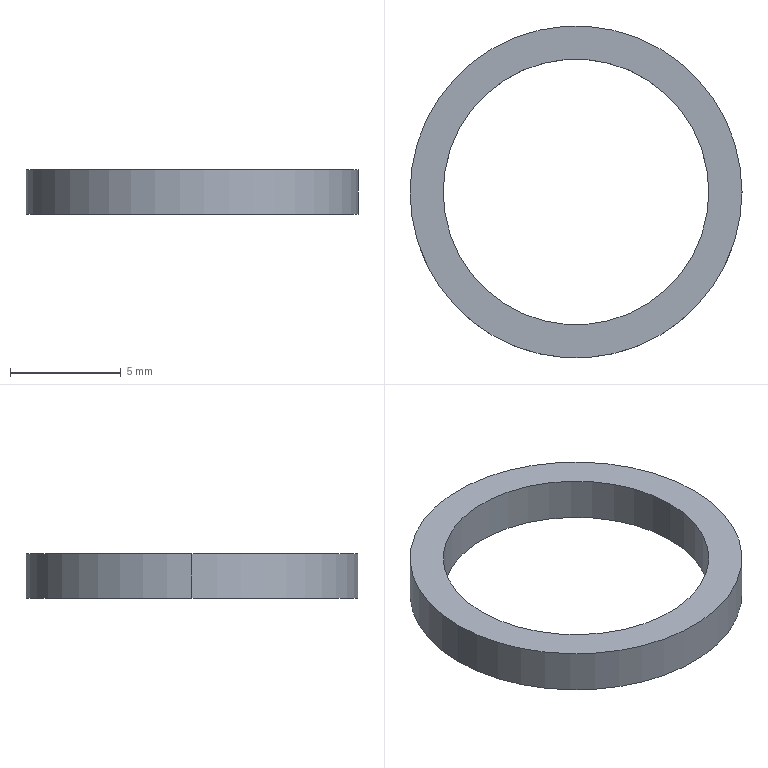Part | SolidWorks | features Extrusion 1 | 1 solid | 6 faces | box 15 x 15 x 2 mm | volume 127.235 mm3 | cylinder 4 | plane 2 | commonest cylinder face diameters 12 x2 15 x2
STEP:
#1=CARTESIAN_POINT('',(-6.,0.,2.));
#2=VERTEX_POINT('',#1);
#3=CARTESIAN_POINT('',(6.,0.,2.));
#4=VERTEX_POINT('',#3);
#5=CARTESIAN_POINT('',(0.,0.,2.));
#6=DIRECTION('',(0.,0.,1.));
#7=DIRECTION('',(1.,0.,0.));
#8=AXIS2_PLACEMENT_3D('',#5,#6,#7);
#9=CIRCLE('',#8,6.);
#10=EDGE_CURVE('',#2,#4,#9,.T.);
#11=ORIENTED_EDGE('',*,*,#10,.T.);
#12=CARTESIAN_POINT('',(6.,0.,0.));
#13=VERTEX_POINT('',#12);
#14=CARTESIAN_POINT('',(6.,0.,2.));
#15=DIRECTION('',(0.,0.,-1.));
#16=VECTOR('',#15,1000.);
#17=LINE('',#14,#16);
#18=EDGE_CURVE('',#4,#13,#17,.T.);
#19=ORIENTED_EDGE('',*,*,#18,.T.);
#20=CARTESIAN_POINT('',(-6.,0.,0.));
#21=VERTEX_POINT('',#20);
#22=CARTESIAN_POINT('',(0.,0.,0.));
#23=DIRECTION('',(0.,0.,1.));
#24=DIRECTION('',(1.,0.,0.));
#25=AXIS2_PLACEMENT_3D('',#22,#23,#24);
#26=CIRCLE('',#25,6.);
#27=EDGE_CURVE('',#21,#13,#26,.T.);
#28=ORIENTED_EDGE('',*,*,#27,.F.);
#29=CARTESIAN_POINT('',(-6.,0.,2.));
#30=DIRECTION('',(0.,0.,-1.));
#31=VECTOR('',#30,1000.);
#32=LINE('',#29,#31);
#33=EDGE_CURVE('',#2,#21,#32,.T.);
#34=ORIENTED_EDGE('',*,*,#33,.F.);
#35=EDGE_LOOP('',(#11,#19,#28,#34));
#36=FACE_OUTER_BOUND('',#35,.T.);
#37=CARTESIAN_POINT('',(0.,0.,2.));
#38=DIRECTION('',(0.,0.,-1.));
#39=DIRECTION('',(-1.,0.,0.));
#40=AXIS2_PLACEMENT_3D('',#37,#38,#39);
#41=CYLINDRICAL_SURFACE('',#40,6.);
#42=ADVANCED_FACE('',(#36),#41,.F.);
#43=CARTESIAN_POINT('',(7.5,0.,2.));
#44=VERTEX_POINT('',#43);
#45=CARTESIAN_POINT('',(-7.5,0.,2.));
#46=VERTEX_POINT('',#45);
#47=CARTESIAN_POINT('',(0.,0.,2.));
#48=DIRECTION('',(0.,0.,1.));
#49=DIRECTION('',(1.,0.,0.));
#50=AXIS2_PLACEMENT_3D('',#47,#48,#49);
#51=CIRCLE('',#50,7.5);
#52=EDGE_CURVE('',#44,#46,#51,.T.);
#53=ORIENTED_EDGE('',*,*,#52,.F.);
#54=CARTESIAN_POINT('',(7.5,0.,0.));
#55=VERTEX_POINT('',#54);
#56=CARTESIAN_POINT('',(7.5,0.,2.));
#57=DIRECTION('',(0.,0.,-1.));
#58=VECTOR('',#57,1000.);
#59=LINE('',#56,#58);
#60=EDGE_CURVE('',#44,#55,#59,.T.);
#61=ORIENTED_EDGE('',*,*,#60,.T.);
#62=CARTESIAN_POINT('',(-7.5,0.,0.));
#63=VERTEX_POINT('',#62);
#64=CARTESIAN_POINT('',(0.,0.,0.));
#65=DIRECTION('',(0.,0.,1.));
#66=DIRECTION('',(1.,0.,0.));
#67=AXIS2_PLACEMENT_3D('',#64,#65,#66);
#68=CIRCLE('',#67,7.5);
#69=EDGE_CURVE('',#55,#63,#68,.T.);
#70=ORIENTED_EDGE('',*,*,#69,.T.);
#71=CARTESIAN_POINT('',(-7.5,0.,2.));
#72=DIRECTION('',(0.,0.,-1.));
#73=VECTOR('',#72,1000.);
#74=LINE('',#71,#73);
#75=EDGE_CURVE('',#46,#63,#74,.T.);
#76=ORIENTED_EDGE('',*,*,#75,.F.);
#77=EDGE_LOOP('',(#53,#61,#70,#76));
#78=FACE_OUTER_BOUND('',#77,.T.);
#79=CARTESIAN_POINT('',(0.,0.,2.));
#80=DIRECTION('',(0.,0.,-1.));
#81=DIRECTION('',(-1.,0.,0.));
#82=AXIS2_PLACEMENT_3D('',#79,#80,#81);
#83=CYLINDRICAL_SURFACE('',#82,7.5);
#84=ADVANCED_FACE('',(#78),#83,.T.);
#85=CARTESIAN_POINT('',(0.,0.,2.));
#86=DIRECTION('',(0.,0.,1.));
#87=DIRECTION('',(1.,0.,0.));
#88=AXIS2_PLACEMENT_3D('',#85,#86,#87);
#89=CIRCLE('',#88,7.5);
#90=EDGE_CURVE('',#46,#44,#89,.T.);
#91=ORIENTED_EDGE('',*,*,#90,.T.);
#92=ORIENTED_EDGE('',*,*,#52,.T.);
#93=EDGE_LOOP('',(#91,#92));
#94=FACE_OUTER_BOUND('',#93,.T.);
#95=ORIENTED_EDGE('',*,*,#10,.F.);
#96=CARTESIAN_POINT('',(0.,0.,2.));
#97=DIRECTION('',(0.,0.,1.));
#98=DIRECTION('',(1.,0.,0.));
#99=AXIS2_PLACEMENT_3D('',#96,#97,#98);
#100=CIRCLE('',#99,6.);
#101=EDGE_CURVE('',#4,#2,#100,.T.);
#102=ORIENTED_EDGE('',*,*,#101,.F.);
#103=EDGE_LOOP('',(#95,#102));
#104=FACE_BOUND('',#103,.T.);
#105=CARTESIAN_POINT('',(0.,0.,2.));
#106=DIRECTION('',(0.,0.,1.));
#107=DIRECTION('',(1.,0.,0.));
#108=AXIS2_PLACEMENT_3D('',#105,#106,#107);
#109=PLANE('',#108);
#110=ADVANCED_FACE('',(#94,#104),#109,.T.);
#111=CARTESIAN_POINT('',(0.,0.,0.));
#112=DIRECTION('',(0.,0.,1.));
#113=DIRECTION('',(1.,0.,0.));
#114=AXIS2_PLACEMENT_3D('',#111,#112,#113);
#115=CIRCLE('',#114,7.5);
#116=EDGE_CURVE('',#63,#55,#115,.T.);
#117=ORIENTED_EDGE('',*,*,#116,.F.);
#118=ORIENTED_EDGE('',*,*,#69,.F.);
#119=EDGE_LOOP('',(#117,#118));
#120=FACE_OUTER_BOUND('',#119,.T.);
#121=ORIENTED_EDGE('',*,*,#27,.T.);
#122=CARTESIAN_POINT('',(0.,0.,0.));
#123=DIRECTION('',(0.,0.,1.));
#124=DIRECTION('',(1.,0.,0.));
#125=AXIS2_PLACEMENT_3D('',#122,#123,#124);
#126=CIRCLE('',#125,6.);
#127=EDGE_CURVE('',#13,#21,#126,.T.);
#128=ORIENTED_EDGE('',*,*,#127,.T.);
#129=EDGE_LOOP('',(#121,#128));
#130=FACE_BOUND('',#129,.T.);
#131=CARTESIAN_POINT('',(0.,0.,0.));
#132=DIRECTION('',(0.,0.,1.));
#133=DIRECTION('',(1.,0.,0.));
#134=AXIS2_PLACEMENT_3D('',#131,#132,#133);
#135=PLANE('',#134);
#136=ADVANCED_FACE('',(#120,#130),#135,.F.);
#137=ORIENTED_EDGE('',*,*,#60,.F.);
#138=ORIENTED_EDGE('',*,*,#90,.F.);
#139=ORIENTED_EDGE('',*,*,#75,.T.);
#140=ORIENTED_EDGE('',*,*,#116,.T.);
#141=EDGE_LOOP('',(#137,#138,#139,#140));
#142=FACE_OUTER_BOUND('',#141,.T.);
#143=CARTESIAN_POINT('',(0.,0.,2.));
#144=DIRECTION('',(0.,0.,-1.));
#145=DIRECTION('',(-1.,0.,0.));
#146=AXIS2_PLACEMENT_3D('',#143,#144,#145);
#147=CYLINDRICAL_SURFACE('',#146,7.5);
#148=ADVANCED_FACE('',(#142),#147,.T.);
#149=ORIENTED_EDGE('',*,*,#18,.F.);
#150=ORIENTED_EDGE('',*,*,#101,.T.);
#151=ORIENTED_EDGE('',*,*,#33,.T.);
#152=ORIENTED_EDGE('',*,*,#127,.F.);
#153=EDGE_LOOP('',(#149,#150,#151,#152));
#154=FACE_OUTER_BOUND('',#153,.T.);
#155=CARTESIAN_POINT('',(0.,0.,2.));
#156=DIRECTION('',(0.,0.,-1.));
#157=DIRECTION('',(-1.,0.,0.));
#158=AXIS2_PLACEMENT_3D('',#155,#156,#157);
#159=CYLINDRICAL_SURFACE('',#158,6.);
#160=ADVANCED_FACE('',(#154),#159,.F.);
#161=CLOSED_SHELL('',(#42,#84,#110,#136,#148,#160));
#162=MANIFOLD_SOLID_BREP('',#161);
#163=CARTESIAN_POINT('',(0.,0.,0.));
#164=DIRECTION('',(0.,0.,1.));
#165=DIRECTION('',(1.,0.,0.));
#166=AXIS2_PLACEMENT_3D('',#163,#164,#165);
#167=(LENGTH_UNIT()NAMED_UNIT(*)SI_UNIT(.MILLI.,.METRE.));
#168=UNCERTAINTY_MEASURE_WITH_UNIT(LENGTH_MEASURE(0.00001),#167,'','');
#169=(NAMED_UNIT(*)PLANE_ANGLE_UNIT()SI_UNIT($,.RADIAN.));
#170=(NAMED_UNIT(*)SI_UNIT($,.STERADIAN.)SOLID_ANGLE_UNIT());
#171=(GEOMETRIC_REPRESENTATION_CONTEXT(3)GLOBAL_UNCERTAINTY_ASSIGNED_CONTEXT((#168))GLOBAL_UNIT_ASSIGNED_CONTEXT((#167,#169,#170))REPRESENTATION_CONTEXT('',''));
#172=ADVANCED_BREP_SHAPE_REPRESENTATION('',(#162,#166),#171);